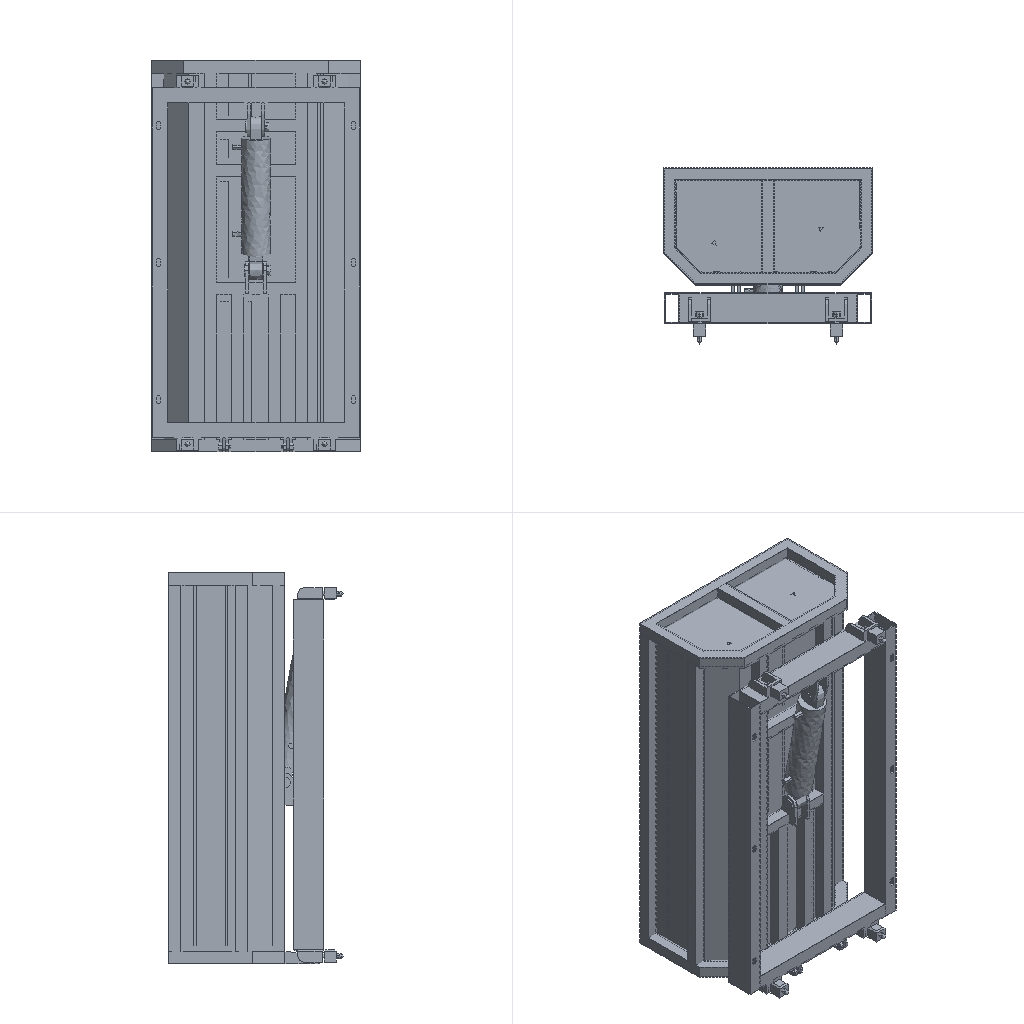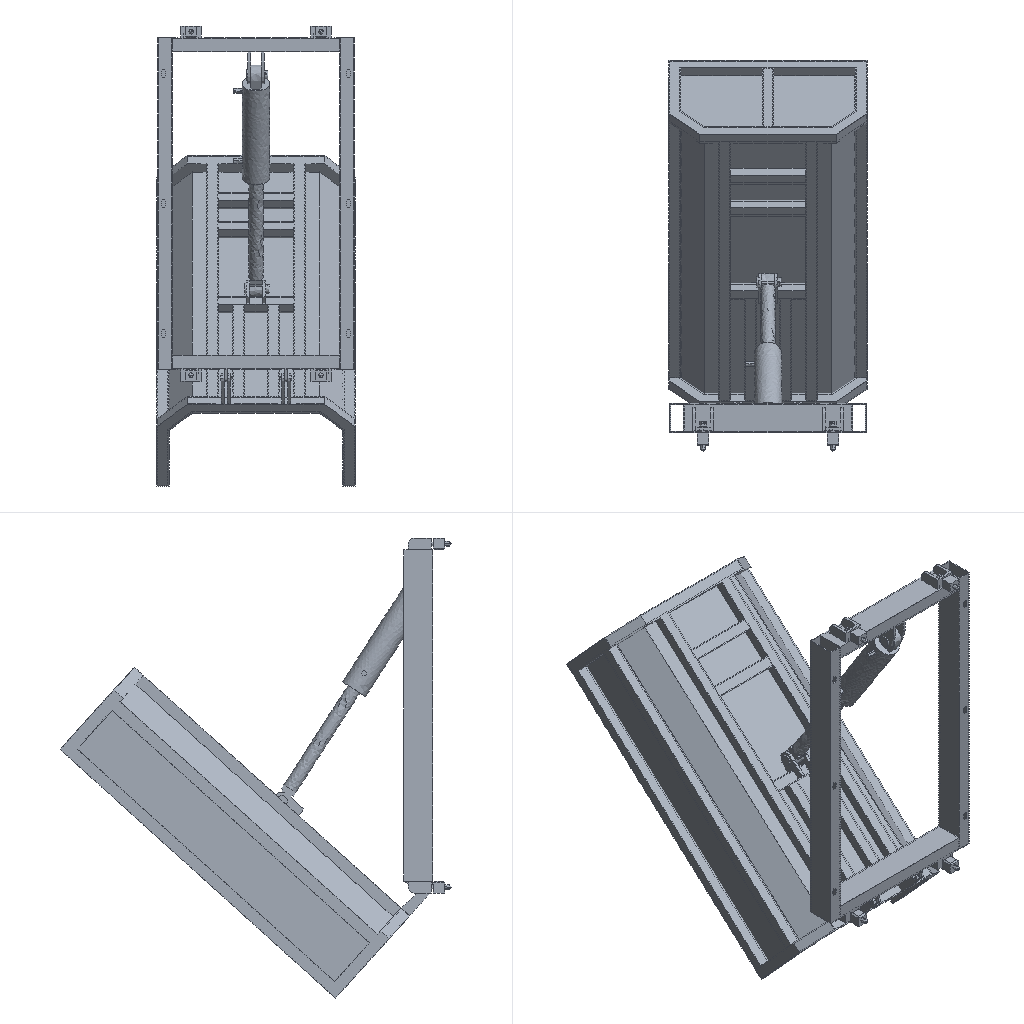Simulation study | ansys workbench
Set-up summary:
category,name,step,type,value,unit,region
solver,ansys_workbench
units,mm-N-s-tonne (MPa),,stated,"/units,MPA"
analysis,deck-1/LS1,,static
load_step,deck-1/LS1,deck-1/LS1,static,nsubst=1; time=1
analysis,deck-2/LS1,,static
load_step,deck-2/LS1,deck-2/LS1,static,nsubst=1; time=1
mesh,deck-1.dat,,nodes,215428
mesh,deck-1.dat,,elements,97787
element_type,SOLID187,,,61849,,deck-1.dat
element_type,SOLID186,,,13476,,deck-1.dat
element_type,TARGE170,,,10892,,deck-1.dat
element_type,CONTA174,,,10892,,deck-1.dat
element_type,SURF154,,,678,,deck-1.dat
mesh,deck-2.dat,,nodes,364808
mesh,deck-2.dat,,elements,189761
element_type,SOLID187,,,127255,,deck-2.dat
element_type,TARGE170,,,19734,,deck-2.dat
element_type,CONTA174,,,19734,,deck-2.dat
element_type,SOLID186,,,15402,,deck-2.dat
element_type,SURF154,,,7636,,deck-2.dat
material,Structural Steel,,E,2e+11,Pa
material,Structural Steel,,nu,0.3
material,Structural Steel,,density,7850,kg m^-3
material,Structural Steel,,conductivity,60.5,W m^-1 C^-1
material,Structural Steel,,specific_heat,434,J kg^-1 C^-1
material,Structural Steel,,cte,1.2e-05,C^-1
material,Structural Steel,,permeability,10000
material,Structural Steel,,resistivity,1.7e-07,kg m^3 A^-2 s^-3
material,Structural Steel,,E,200000,tonne s^-2 mm^-1
material,Structural Steel,,nu,0.3
material,Structural Steel,,density,7.85e-09,tonne mm^-3
material,Structural Steel,,conductivity,60.5,tonne mm s^-3 C^-1
material,Structural Steel,,specific_heat,4.34e+08,mm^2 s^-2 C^-1
material,Structural Steel,,cte,1.2e-05,C^-1
material,Structural Steel,,permeability,10000
material,Structural Steel,,resistivity,0.00017,ohm mm
load,Define Force Using Surface Effect Elements,deck-1/LS1,surface-effect pres face 3,5960.11,,SURF154 #197
load,Define Force Using Surface Effect Elements,deck-2/LS1,surface-effect pres face 2,-0.006042,,SURF154 #157
load,Define Force Using Surface Effect Elements,deck-2/LS1,surface-effect pres face 3,5.18931e-35,,SURF154 #157
bc,Fixed Supports,deck-1/model,fixed,[dofs=ALL],,_FIXEDSU
bc,Fixed Supports,deck-2/model,fixed,[dofs=ALL],,_FIXEDSU
contact,Contact Region,,bonded (always),element=CONTA174
contact,Contact Region 2,,bonded (always),element=CONTA174
contact,Contact Region 3,,bonded (always),element=CONTA174
contact,Contact Region 4,,bonded (always),element=CONTA174
contact,Contact Region 5,,bonded (always),element=CONTA174
contact,Contact Region 6,,bonded (always),element=CONTA174
contact,Contact Region 7,,bonded (always),element=CONTA174
contact,Contact Region 8,,bonded (always),element=CONTA174
contact,Contact Region 10,,bonded (always),element=CONTA174
contact,Contact Region 11,,bonded (always),element=CONTA174
contact,Contact Region 12,,bonded (always),element=CONTA174
contact,Contact Region 13,,bonded (always),element=CONTA174
contact,Contact Region 14,,bonded (always),element=CONTA174
contact,Contact Region 15,,bonded (always),element=CONTA174
contact,Contact Region 16,,bonded (always),element=CONTA174
contact,Contact Region 17,,bonded (always),element=CONTA174
contact,Contact Region 18,,bonded (always),element=CONTA174
contact,Contact Region 19,,bonded (always),element=CONTA174
contact,Contact Region 20,,bonded (always),element=CONTA174
contact,Contact Region 21,,bonded (always),element=CONTA174
contact,Contact Region 22,,bonded (always),element=CONTA174
contact,Contact Region 23,,bonded (always),element=CONTA174
contact,Contact Region 24,,bonded (always),element=CONTA174
contact,Contact Region 25,,bonded (always),element=CONTA174
contact,Contact Region 26,,bonded (always),element=CONTA174
contact,Contact Region 27,,bonded (always),element=CONTA174
contact,Contact Region 28,,bonded (always),element=CONTA174
contact,Contact Region 29,,bonded (always),element=CONTA174
contact,Contact Region 30,,bonded (always),element=CONTA174
contact,Contact Region 32,,bonded (always),element=CONTA174
contact,Contact Region 34,,bonded (always),element=CONTA174
contact,Contact Region 36,,bonded (always),element=CONTA174
contact,Contact Region 38,,bonded (always),element=CONTA174
contact,Contact Region 39,,bonded (always),element=CONTA174
contact,Contact Region 40,,bonded (always),element=CONTA174
contact,Contact Region 42,,bonded (always),element=CONTA174
contact,Contact Region 43,,bonded (always),element=CONTA174
contact,Contact Region 45,,bonded (always),element=CONTA174
contact,Contact Region 46,,bonded (always),element=CONTA174
contact,Contact Region 47,,bonded (always),element=CONTA174
contact,Contact Region 48,,bonded (always),element=CONTA174
contact,Contact Region 49,,bonded (always),element=CONTA174
contact,Contact Region 50,,bonded (always),element=CONTA174
contact,Contact Region 51,,bonded (always),element=CONTA174
contact,Contact Region 52,,bonded (always),element=CONTA174
contact,Contact Region 53,,bonded (always),element=CONTA174
contact,Contact Region 54,,bonded (always),element=CONTA174
contact,Contact Region 55,,bonded (always),element=CONTA174
contact,Contact Region 56,,bonded (always),element=CONTA174
contact,Contact Region 57,,bonded (always),element=CONTA174
contact,Contact Region 58,,bonded (always),element=CONTA174
contact,Contact Region 59,,bonded (always),element=CONTA174
contact,Contact Region 60,,bonded (always),element=CONTA174
contact,Contact Region 61,,bonded (always),element=CONTA174
contact,Contact Region 62,,bonded (always),element=CONTA174
contact,Contact Region 63,,bonded (always),element=CONTA174
contact,Contact Region 64,,bonded (always),element=CONTA174
contact,Contact Region 65,,bonded (always),element=CONTA174
contact,Contact Region 66,,bonded (always),element=CONTA174
contact,Contact Region 67,,bonded (always),element=CONTA174
contact,Contact Region 68,,bonded (always),element=CONTA174
contact,Contact Region 69,,bonded (always),element=CONTA174
contact,Contact Region 70,,bonded (always),element=CONTA174
contact,Contact Region 71,,bonded (always),element=CONTA174
contact,Contact Region 72,,bonded (always),element=CONTA174
contact,Contact Region 73,,bonded (always),element=CONTA174
contact,Contact Region 76,,bonded (always),element=CONTA174
contact,Contact Region 77,,bonded (always),element=CONTA174
contact,Contact Region 78,,bonded (always),element=CONTA174
contact,Contact Region 79,,bonded (always),element=CONTA174
contact,Contact Region 80,,bonded (always),element=CONTA174
contact,Contact Region 81,,bonded (always),element=CONTA174
contact,Contact Region 82,,bonded (always),element=CONTA174
contact,Contact Region 83,,bonded (always),element=CONTA174
contact,Bonded - gangtong\____-____3 ? ?28?250\____-____2,,bonded (always),element=CONTA174
contact,Contact Region,,bonded (always),element=CONTA174
contact,Contact Region 2,,bonded (always),element=CONTA174
contact,Contact Region 3,,bonded (always),element=CONTA174
contact,Contact Region 6,,bonded (always),element=CONTA174
contact,Contact Region 7,,bonded (always),element=CONTA174
contact,Contact Region 8,,bonded (always),element=CONTA174
contact,Contact Region 9,,bonded (always),element=CONTA174
contact,Contact Region 10,,bonded (always),element=CONTA174
contact,Contact Region 11,,bonded (always),element=CONTA174
contact,Contact Region 12,,bonded (always),element=CONTA174
contact,Contact Region 13,,bonded (always),element=CONTA174
contact,Contact Region 15,,bonded (always),element=CONTA174
contact,Contact Region 17,,bonded (always),element=CONTA174
contact,Contact Region 19,,bonded (always),element=CONTA174
contact,Contact Region 21,,bonded (always),element=CONTA174
contact,Contact Region 22,,bonded (always),element=CONTA174
contact,Contact Region 23,,bonded (always),element=CONTA174
contact,Contact Region 25,,bonded (always),element=CONTA174
contact,Contact Region 26,,bonded (always),element=CONTA174
contact,Contact Region 28,,bonded (always),element=CONTA174
contact,Contact Region 29,,bonded (always),element=CONTA174
contact,Contact Region 30,,bonded (always),element=CONTA174
contact,Contact Region 31,,bonded (always),element=CONTA174
contact,Contact Region 32,,bonded (always),element=CONTA174
contact,Contact Region 33,,bonded (always),element=CONTA174
contact,Contact Region 34,,bonded (always),element=CONTA174
contact,Contact Region 35,,bonded (always),element=CONTA174
contact,Contact Region 36,,bonded (always),element=CONTA174
contact,Contact Region 37,,bonded (always),element=CONTA174
contact,Contact Region 38,,bonded (always),element=CONTA174
contact,Contact Region 39,,bonded (always),element=CONTA174
contact,Contact Region 40,,bonded (always),element=CONTA174
contact,Contact Region 41,,bonded (always),element=CONTA174
contact,Contact Region 42,,bonded (always),element=CONTA174
contact,Contact Region 43,,bonded (always),element=CONTA174
contact,Contact Region 44,,bonded (always),element=CONTA174
contact,Contact Region 45,,bonded (always),element=CONTA174
contact,Contact Region 46,,bonded (always),element=CONTA174
contact,Contact Region 47,,bonded (always),element=CONTA174
contact,Contact Region 48,,bonded (always),element=CONTA174
contact,Contact Region 49,,bonded (always),element=CONTA174
contact,Contact Region 50,,bonded (always),element=CONTA174
contact,Contact Region 51,,bonded (always),element=CONTA174
contact,Contact Region 52,,bonded (always),element=CONTA174
contact,Contact Region 53,,bonded (always),element=CONTA174
contact,Contact Region 54,,bonded (always),element=CONTA174
contact,Contact Region 55,,bonded (always),element=CONTA174
contact,Contact Region 56,,bonded (always),element=CONTA174
contact,Contact Region 57,,bonded (always),element=CONTA174
contact,Contact Region 58,,bonded (always),element=CONTA174
contact,Contact Region 59,,bonded (always),element=CONTA174
contact,Contact Region 60,,bonded (always),element=CONTA174
contact,Contact Region 61,,bonded (always),element=CONTA174
contact,Contact Region 62,,bonded (always),element=CONTA174
contact,Contact Region 63,,bonded (always),element=CONTA174
contact,Contact Region 64,,bonded (always),element=CONTA174
contact,Contact Region 65,,bonded (always),element=CONTA174
contact,Contact Region 66,,bonded (always),element=CONTA174
named_set,_FIXEDSU,,node,84
named_set,_FIXEDSU,,node,148
Results summary:
result,analyses[0].index,,,1
result,analyses[0].system,,,SYS
result,analyses[0].deck,,,deck-1.dat
result,analyses[0].solve_status,,,completed
result,analyses[0].analysis_type,,,static
result,analyses[0].physics,,,mechanical
result,analyses[0].unit_system,,,"MKS: m, kg, N, s, V, A, degC"
result,analyses[0].n_sets,,,1
result,analyses[0].load_steps[0].set,set=1,,1
result,analyses[0].load_steps[0].time_or_freq,set=1,,1
result,analyses[0].load_steps[0].max_displacement_magnitude,set=1,,0.0004086
result,analyses[0].load_steps[0].max_von_mises_nodal,set=1,,8.9314e+07
result,analyses[0].load_steps[0].reaction_force_sum_xyz[1],set=1,,2.68087e-05
result,analyses[0].load_steps[0].reaction_force_sum_xyz[2],set=1,,-3.93221e-06
result,analyses[0].load_steps[0].reaction_force_sum_xyz[3],set=1,,-1500
result,analyses[1].index,,,2
result,analyses[1].system,,,SYS-1
result,analyses[1].deck,,,deck-2.dat
result,analyses[1].solve_status,,,completed
result,analyses[1].analysis_type,,,static
result,analyses[1].physics,,,mechanical
result,analyses[1].unit_system,,,"NMM: mm, ton, N, s, mV, mA, degC"
result,analyses[1].n_sets,,,1
result,analyses[1].load_steps[0].set,set=1,,1
result,analyses[1].load_steps[0].time_or_freq,set=1,,1
result,analyses[1].load_steps[0].max_displacement_magnitude,set=1,,0.7898
result,analyses[1].load_steps[0].max_von_mises_nodal,set=1,,106.689
result,analyses[1].load_steps[0].reaction_force_sum_xyz[1],set=1,,-6.78718e-06
result,analyses[1].load_steps[0].reaction_force_sum_xyz[2],set=1,,5000
result,analyses[1].load_steps[0].reaction_force_sum_xyz[3],set=1,,-1.03348e-05
result,geometry_export[0][0],,,1.step
result,geometry_export[0][1],,,ok
result,geometry_export[0][2],,,46
result,geometry_export[1][0],,,2.step
result,geometry_export[1][1],,,ok
result,geometry_export[1][2],,,40